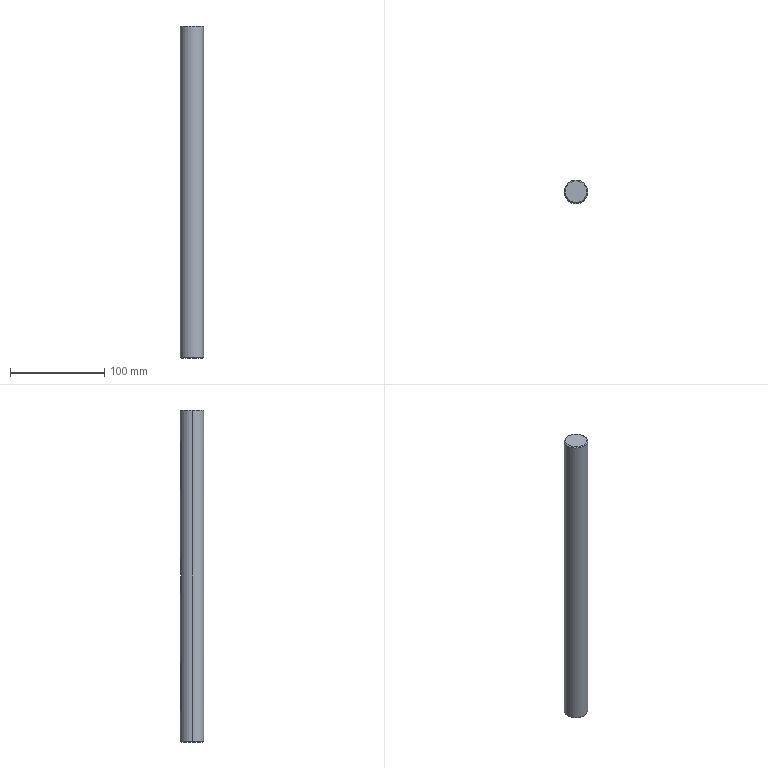Part | 1 solid | 35 faces | box 25 x 25 x 353 mm | volume 169122 mm3 | plane 17 | cylinder 14 | cone 4 | commonest cylinder face diameters 0.6 x12 25 x2
STEP:
#1=CARTESIAN_POINT('',(11.5,0.,176.5));
#2=VERTEX_POINT('',#1);
#3=CARTESIAN_POINT('',(-11.5,0.,176.5));
#4=VERTEX_POINT('',#3);
#5=CARTESIAN_POINT('',(0.,0.,176.5));
#6=DIRECTION('',(0.,0.,1.));
#7=DIRECTION('',(1.,0.,0.));
#8=AXIS2_PLACEMENT_3D('',#5,#6,#7);
#9=CIRCLE('',#8,11.5);
#10=EDGE_CURVE('',#2,#4,#9,.T.);
#11=ORIENTED_EDGE('',*,*,#10,.F.);
#12=CARTESIAN_POINT('',(12.5,0.,175.5));
#13=VERTEX_POINT('',#12);
#14=CARTESIAN_POINT('',(11.5,0.,176.5));
#15=DIRECTION('',(0.7071,0.,-0.7071));
#16=VECTOR('',#15,1000.);
#17=LINE('',#14,#16);
#18=EDGE_CURVE('',#2,#13,#17,.T.);
#19=ORIENTED_EDGE('',*,*,#18,.T.);
#20=CARTESIAN_POINT('',(-12.5,0.,175.5));
#21=VERTEX_POINT('',#20);
#22=CARTESIAN_POINT('',(0.,0.,175.5));
#23=DIRECTION('',(0.,0.,-1.));
#24=DIRECTION('',(1.,0.,0.));
#25=AXIS2_PLACEMENT_3D('',#22,#23,#24);
#26=CIRCLE('',#25,12.5);
#27=EDGE_CURVE('',#21,#13,#26,.T.);
#28=ORIENTED_EDGE('',*,*,#27,.F.);
#29=CARTESIAN_POINT('',(-11.5,0.,176.5));
#30=DIRECTION('',(-0.7071,0.,-0.7071));
#31=VECTOR('',#30,1000.);
#32=LINE('',#29,#31);
#33=EDGE_CURVE('',#4,#21,#32,.T.);
#34=ORIENTED_EDGE('',*,*,#33,.F.);
#35=EDGE_LOOP('',(#11,#19,#28,#34));
#36=FACE_OUTER_BOUND('',#35,.T.);
#37=CARTESIAN_POINT('',(0.,0.,176.5));
#38=DIRECTION('',(0.,0.,-1.));
#39=DIRECTION('',(-1.,0.,0.));
#40=AXIS2_PLACEMENT_3D('',#37,#38,#39);
#41=CONICAL_SURFACE('',#40,11.5,0.7854);
#42=ADVANCED_FACE('',(#36),#41,.T.);
#43=CARTESIAN_POINT('',(-11.5,0.,-176.5));
#44=VERTEX_POINT('',#43);
#45=CARTESIAN_POINT('',(11.5,0.,-176.5));
#46=VERTEX_POINT('',#45);
#47=CARTESIAN_POINT('',(0.,0.,-176.5));
#48=DIRECTION('',(0.,0.,-1.));
#49=DIRECTION('',(1.,0.,0.));
#50=AXIS2_PLACEMENT_3D('',#47,#48,#49);
#51=CIRCLE('',#50,11.5);
#52=EDGE_CURVE('',#44,#46,#51,.T.);
#53=ORIENTED_EDGE('',*,*,#52,.F.);
#54=CARTESIAN_POINT('',(-12.5,0.,-175.5));
#55=VERTEX_POINT('',#54);
#56=CARTESIAN_POINT('',(-12.5,0.,-175.5));
#57=DIRECTION('',(-0.7071,0.,0.7071));
#58=VECTOR('',#57,1000.);
#59=LINE('',#56,#58);
#60=EDGE_CURVE('',#44,#55,#59,.T.);
#61=ORIENTED_EDGE('',*,*,#60,.T.);
#62=CARTESIAN_POINT('',(12.5,0.,-175.5));
#63=VERTEX_POINT('',#62);
#64=CARTESIAN_POINT('',(0.,0.,-175.5));
#65=DIRECTION('',(0.,0.,1.));
#66=DIRECTION('',(1.,0.,0.));
#67=AXIS2_PLACEMENT_3D('',#64,#65,#66);
#68=CIRCLE('',#67,12.5);
#69=EDGE_CURVE('',#63,#55,#68,.T.);
#70=ORIENTED_EDGE('',*,*,#69,.F.);
#71=CARTESIAN_POINT('',(12.5,0.,-175.5));
#72=DIRECTION('',(0.7071,0.,0.7071));
#73=VECTOR('',#72,1000.);
#74=LINE('',#71,#73);
#75=EDGE_CURVE('',#46,#63,#74,.T.);
#76=ORIENTED_EDGE('',*,*,#75,.F.);
#77=EDGE_LOOP('',(#53,#61,#70,#76));
#78=FACE_OUTER_BOUND('',#77,.T.);
#79=CARTESIAN_POINT('',(0.,0.,-175.5));
#80=DIRECTION('',(0.,0.,1.));
#81=DIRECTION('',(1.,0.,0.));
#82=AXIS2_PLACEMENT_3D('',#79,#80,#81);
#83=CONICAL_SURFACE('',#82,12.5,0.7854);
#84=ADVANCED_FACE('',(#78),#83,.T.);
#85=CARTESIAN_POINT('',(-4.,11.843,143.5));
#86=VERTEX_POINT('',#85);
#87=CARTESIAN_POINT('',(-4.,11.843,93.5));
#88=VERTEX_POINT('',#87);
#89=CARTESIAN_POINT('',(-4.,11.843,176.5));
#90=DIRECTION('',(0.,0.,-1.));
#91=VECTOR('',#90,1000.);
#92=LINE('',#89,#91);
#93=EDGE_CURVE('',#86,#88,#92,.T.);
#94=ORIENTED_EDGE('',*,*,#93,.T.);
#95=CARTESIAN_POINT('',(4.,11.843,93.5));
#96=VERTEX_POINT('',#95);
#97=CARTESIAN_POINT('',(0.,0.,93.5));
#98=DIRECTION('',(0.,0.,-1.));
#99=DIRECTION('',(-1.,0.,0.));
#100=AXIS2_PLACEMENT_3D('',#97,#98,#99);
#101=CIRCLE('',#100,12.5);
#102=EDGE_CURVE('',#88,#96,#101,.T.);
#103=ORIENTED_EDGE('',*,*,#102,.T.);
#104=CARTESIAN_POINT('',(4.,11.843,143.5));
#105=VERTEX_POINT('',#104);
#106=CARTESIAN_POINT('',(4.,11.843,176.5));
#107=DIRECTION('',(0.,0.,1.));
#108=VECTOR('',#107,1000.);
#109=LINE('',#106,#108);
#110=EDGE_CURVE('',#96,#105,#109,.T.);
#111=ORIENTED_EDGE('',*,*,#110,.T.);
#112=CARTESIAN_POINT('',(0.,0.,143.5));
#113=DIRECTION('',(0.,0.,1.));
#114=DIRECTION('',(1.,0.,0.));
#115=AXIS2_PLACEMENT_3D('',#112,#113,#114);
#116=CIRCLE('',#115,12.5);
#117=EDGE_CURVE('',#105,#86,#116,.T.);
#118=ORIENTED_EDGE('',*,*,#117,.T.);
#119=EDGE_LOOP('',(#94,#103,#111,#118));
#120=FACE_BOUND('',#119,.T.);
#121=CARTESIAN_POINT('',(4.,11.843,-143.5));
#122=VERTEX_POINT('',#121);
#123=CARTESIAN_POINT('',(4.,11.843,-93.5));
#124=VERTEX_POINT('',#123);
#125=CARTESIAN_POINT('',(4.,11.843,176.5));
#126=DIRECTION('',(0.,0.,1.));
#127=VECTOR('',#126,1000.);
#128=LINE('',#125,#127);
#129=EDGE_CURVE('',#122,#124,#128,.T.);
#130=ORIENTED_EDGE('',*,*,#129,.T.);
#131=CARTESIAN_POINT('',(-4.,11.843,-93.5));
#132=VERTEX_POINT('',#131);
#133=CARTESIAN_POINT('',(0.,0.,-93.5));
#134=DIRECTION('',(0.,0.,1.));
#135=DIRECTION('',(1.,0.,0.));
#136=AXIS2_PLACEMENT_3D('',#133,#134,#135);
#137=CIRCLE('',#136,12.5);
#138=EDGE_CURVE('',#124,#132,#137,.T.);
#139=ORIENTED_EDGE('',*,*,#138,.T.);
#140=CARTESIAN_POINT('',(-4.,11.843,-143.5));
#141=VERTEX_POINT('',#140);
#142=CARTESIAN_POINT('',(-4.,11.843,176.5));
#143=DIRECTION('',(0.,0.,-1.));
#144=VECTOR('',#143,1000.);
#145=LINE('',#142,#144);
#146=EDGE_CURVE('',#132,#141,#145,.T.);
#147=ORIENTED_EDGE('',*,*,#146,.T.);
#148=CARTESIAN_POINT('',(0.,0.,-143.5));
#149=DIRECTION('',(0.,0.,-1.));
#150=DIRECTION('',(-1.,0.,0.));
#151=AXIS2_PLACEMENT_3D('',#148,#149,#150);
#152=CIRCLE('',#151,12.5);
#153=EDGE_CURVE('',#141,#122,#152,.T.);
#154=ORIENTED_EDGE('',*,*,#153,.T.);
#155=EDGE_LOOP('',(#130,#139,#147,#154));
#156=FACE_BOUND('',#155,.T.);
#157=CARTESIAN_POINT('',(4.,11.843,-17.5));
#158=VERTEX_POINT('',#157);
#159=CARTESIAN_POINT('',(4.,11.843,17.5));
#160=VERTEX_POINT('',#159);
#161=CARTESIAN_POINT('',(4.,11.843,176.5));
#162=DIRECTION('',(0.,0.,1.));
#163=VECTOR('',#162,1000.);
#164=LINE('',#161,#163);
#165=EDGE_CURVE('',#158,#160,#164,.T.);
#166=ORIENTED_EDGE('',*,*,#165,.T.);
#167=CARTESIAN_POINT('',(-4.,11.843,17.5));
#168=VERTEX_POINT('',#167);
#169=CARTESIAN_POINT('',(0.,0.,17.5));
#170=DIRECTION('',(0.,0.,1.));
#171=DIRECTION('',(1.,0.,0.));
#172=AXIS2_PLACEMENT_3D('',#169,#170,#171);
#173=CIRCLE('',#172,12.5);
#174=EDGE_CURVE('',#160,#168,#173,.T.);
#175=ORIENTED_EDGE('',*,*,#174,.T.);
#176=CARTESIAN_POINT('',(-4.,11.843,-17.5));
#177=VERTEX_POINT('',#176);
#178=CARTESIAN_POINT('',(-4.,11.843,176.5));
#179=DIRECTION('',(0.,0.,-1.));
#180=VECTOR('',#179,1000.);
#181=LINE('',#178,#180);
#182=EDGE_CURVE('',#168,#177,#181,.T.);
#183=ORIENTED_EDGE('',*,*,#182,.T.);
#184=CARTESIAN_POINT('',(0.,0.,-17.5));
#185=DIRECTION('',(0.,0.,-1.));
#186=DIRECTION('',(-1.,0.,0.));
#187=AXIS2_PLACEMENT_3D('',#184,#185,#186);
#188=CIRCLE('',#187,12.5);
#189=EDGE_CURVE('',#177,#158,#188,.T.);
#190=ORIENTED_EDGE('',*,*,#189,.T.);
#191=EDGE_LOOP('',(#166,#175,#183,#190));
#192=FACE_BOUND('',#191,.T.);
#193=ORIENTED_EDGE('',*,*,#27,.T.);
#194=CARTESIAN_POINT('',(12.5,0.,176.5));
#195=DIRECTION('',(0.,0.,-1.));
#196=VECTOR('',#195,1000.);
#197=LINE('',#194,#196);
#198=EDGE_CURVE('',#13,#63,#197,.T.);
#199=ORIENTED_EDGE('',*,*,#198,.T.);
#200=ORIENTED_EDGE('',*,*,#69,.T.);
#201=CARTESIAN_POINT('',(-12.5,0.,176.5));
#202=DIRECTION('',(0.,0.,-1.));
#203=VECTOR('',#202,1000.);
#204=LINE('',#201,#203);
#205=EDGE_CURVE('',#21,#55,#204,.T.);
#206=ORIENTED_EDGE('',*,*,#205,.F.);
#207=EDGE_LOOP('',(#193,#199,#200,#206));
#208=FACE_OUTER_BOUND('',#207,.T.);
#209=CARTESIAN_POINT('',(0.,0.,176.5));
#210=DIRECTION('',(0.,0.,-1.));
#211=DIRECTION('',(-1.,0.,0.));
#212=AXIS2_PLACEMENT_3D('',#209,#210,#211);
#213=CYLINDRICAL_SURFACE('',#212,12.5);
#214=ADVANCED_FACE('',(#120,#156,#192,#208),#213,.T.);
#215=ORIENTED_EDGE('',*,*,#198,.F.);
#216=CARTESIAN_POINT('',(0.,0.,175.5));
#217=DIRECTION('',(0.,0.,-1.));
#218=DIRECTION('',(1.,0.,0.));
#219=AXIS2_PLACEMENT_3D('',#216,#217,#218);
#220=CIRCLE('',#219,12.5);
#221=EDGE_CURVE('',#13,#21,#220,.T.);
#222=ORIENTED_EDGE('',*,*,#221,.T.);
#223=ORIENTED_EDGE('',*,*,#205,.T.);
#224=CARTESIAN_POINT('',(0.,0.,-175.5));
#225=DIRECTION('',(0.,0.,1.));
#226=DIRECTION('',(1.,0.,0.));
#227=AXIS2_PLACEMENT_3D('',#224,#225,#226);
#228=CIRCLE('',#227,12.5);
#229=EDGE_CURVE('',#55,#63,#228,.T.);
#230=ORIENTED_EDGE('',*,*,#229,.T.);
#231=EDGE_LOOP('',(#215,#222,#223,#230));
#232=FACE_OUTER_BOUND('',#231,.T.);
#233=CARTESIAN_POINT('',(0.,0.,176.5));
#234=DIRECTION('',(0.,0.,-1.));
#235=DIRECTION('',(-1.,0.,0.));
#236=AXIS2_PLACEMENT_3D('',#233,#234,#235);
#237=CYLINDRICAL_SURFACE('',#236,12.5);
#238=ADVANCED_FACE('',(#232),#237,.T.);
#239=CARTESIAN_POINT('',(0.,0.,176.5));
#240=DIRECTION('',(0.,0.,1.));
#241=DIRECTION('',(1.,0.,0.));
#242=AXIS2_PLACEMENT_3D('',#239,#240,#241);
#243=CIRCLE('',#242,11.5);
#244=EDGE_CURVE('',#4,#2,#243,.T.);
#245=ORIENTED_EDGE('',*,*,#244,.T.);
#246=ORIENTED_EDGE('',*,*,#10,.T.);
#247=EDGE_LOOP('',(#245,#246));
#248=FACE_OUTER_BOUND('',#247,.T.);
#249=CARTESIAN_POINT('',(0.,0.,176.5));
#250=DIRECTION('',(0.,0.,1.));
#251=DIRECTION('',(1.,0.,0.));
#252=AXIS2_PLACEMENT_3D('',#249,#250,#251);
#253=PLANE('',#252);
#254=ADVANCED_FACE('',(#248),#253,.T.);
#255=CARTESIAN_POINT('',(0.,0.,-176.5));
#256=DIRECTION('',(0.,0.,-1.));
#257=DIRECTION('',(1.,0.,0.));
#258=AXIS2_PLACEMENT_3D('',#255,#256,#257);
#259=CIRCLE('',#258,11.5);
#260=EDGE_CURVE('',#46,#44,#259,.T.);
#261=ORIENTED_EDGE('',*,*,#260,.T.);
#262=ORIENTED_EDGE('',*,*,#52,.T.);
#263=EDGE_LOOP('',(#261,#262));
#264=FACE_OUTER_BOUND('',#263,.T.);
#265=CARTESIAN_POINT('',(0.,0.,-176.5));
#266=DIRECTION('',(0.,0.,1.));
#267=DIRECTION('',(1.,0.,0.));
#268=AXIS2_PLACEMENT_3D('',#265,#266,#267);
#269=PLANE('',#268);
#270=ADVANCED_FACE('',(#264),#269,.F.);
#271=CARTESIAN_POINT('',(-4.,8.8,17.5));
#272=VERTEX_POINT('',#271);
#273=CARTESIAN_POINT('',(-4.,8.5,17.5));
#274=DIRECTION('',(0.,1.,0.));
#275=VECTOR('',#274,1000.);
#276=LINE('',#273,#275);
#277=EDGE_CURVE('',#272,#168,#276,.T.);
#278=ORIENTED_EDGE('',*,*,#277,.F.);
#279=CARTESIAN_POINT('',(-4.,8.8,-17.5));
#280=VERTEX_POINT('',#279);
#281=CARTESIAN_POINT('',(-4.,8.8,-17.5));
#282=DIRECTION('',(0.,0.,-1.));
#283=VECTOR('',#282,1000.);
#284=LINE('',#281,#283);
#285=EDGE_CURVE('',#272,#280,#284,.T.);
#286=ORIENTED_EDGE('',*,*,#285,.T.);
#287=CARTESIAN_POINT('',(-4.,8.5,-17.5));
#288=DIRECTION('',(0.,1.,0.));
#289=VECTOR('',#288,1000.);
#290=LINE('',#287,#289);
#291=EDGE_CURVE('',#280,#177,#290,.T.);
#292=ORIENTED_EDGE('',*,*,#291,.T.);
#293=ORIENTED_EDGE('',*,*,#182,.F.);
#294=EDGE_LOOP('',(#278,#286,#292,#293));
#295=FACE_OUTER_BOUND('',#294,.T.);
#296=CARTESIAN_POINT('',(-4.,8.5,-17.5));
#297=DIRECTION('',(-1.,0.,0.));
#298=DIRECTION('',(0.,0.,1.));
#299=AXIS2_PLACEMENT_3D('',#296,#297,#298);
#300=PLANE('',#299);
#301=ADVANCED_FACE('',(#295),#300,.F.);
#302=ORIENTED_EDGE('',*,*,#291,.F.);
#303=CARTESIAN_POINT('',(4.,8.8,-17.5));
#304=VERTEX_POINT('',#303);
#305=CARTESIAN_POINT('',(-4.,8.8,-17.5));
#306=DIRECTION('',(1.,0.,0.));
#307=VECTOR('',#306,1000.);
#308=LINE('',#305,#307);
#309=EDGE_CURVE('',#280,#304,#308,.T.);
#310=ORIENTED_EDGE('',*,*,#309,.T.);
#311=CARTESIAN_POINT('',(4.,8.5,-17.5));
#312=DIRECTION('',(0.,1.,0.));
#313=VECTOR('',#312,1000.);
#314=LINE('',#311,#313);
#315=EDGE_CURVE('',#304,#158,#314,.T.);
#316=ORIENTED_EDGE('',*,*,#315,.T.);
#317=ORIENTED_EDGE('',*,*,#189,.F.);
#318=EDGE_LOOP('',(#302,#310,#316,#317));
#319=FACE_OUTER_BOUND('',#318,.T.);
#320=CARTESIAN_POINT('',(-4.,8.5,-17.5));
#321=DIRECTION('',(0.,0.,-1.));
#322=DIRECTION('',(-1.,0.,0.));
#323=AXIS2_PLACEMENT_3D('',#320,#321,#322);
#324=PLANE('',#323);
#325=ADVANCED_FACE('',(#319),#324,.F.);
#326=ORIENTED_EDGE('',*,*,#315,.F.);
#327=CARTESIAN_POINT('',(4.,8.8,17.5));
#328=VERTEX_POINT('',#327);
#329=CARTESIAN_POINT('',(4.,8.8,-17.5));
#330=DIRECTION('',(0.,0.,1.));
#331=VECTOR('',#330,1000.);
#332=LINE('',#329,#331);
#333=EDGE_CURVE('',#304,#328,#332,.T.);
#334=ORIENTED_EDGE('',*,*,#333,.T.);
#335=CARTESIAN_POINT('',(4.,8.5,17.5));
#336=DIRECTION('',(0.,1.,0.));
#337=VECTOR('',#336,1000.);
#338=LINE('',#335,#337);
#339=EDGE_CURVE('',#328,#160,#338,.T.);
#340=ORIENTED_EDGE('',*,*,#339,.T.);
#341=ORIENTED_EDGE('',*,*,#165,.F.);
#342=EDGE_LOOP('',(#326,#334,#340,#341));
#343=FACE_OUTER_BOUND('',#342,.T.);
#344=CARTESIAN_POINT('',(4.,8.5,-17.5));
#345=DIRECTION('',(1.,0.,0.));
#346=DIRECTION('',(0.,0.,-1.));
#347=AXIS2_PLACEMENT_3D('',#344,#345,#346);
#348=PLANE('',#347);
#349=ADVANCED_FACE('',(#343),#348,.F.);
#350=ORIENTED_EDGE('',*,*,#339,.F.);
#351=CARTESIAN_POINT('',(-4.,8.8,17.5));
#352=DIRECTION('',(-1.,0.,0.));
#353=VECTOR('',#352,1000.);
#354=LINE('',#351,#353);
#355=EDGE_CURVE('',#328,#272,#354,.T.);
#356=ORIENTED_EDGE('',*,*,#355,.T.);
#357=ORIENTED_EDGE('',*,*,#277,.T.);
#358=ORIENTED_EDGE('',*,*,#174,.F.);
#359=EDGE_LOOP('',(#350,#356,#357,#358));
#360=FACE_OUTER_BOUND('',#359,.T.);
#361=CARTESIAN_POINT('',(-4.,8.5,17.5));
#362=DIRECTION('',(0.,0.,1.));
#363=DIRECTION('',(1.,0.,0.));
#364=AXIS2_PLACEMENT_3D('',#361,#362,#363);
#365=PLANE('',#364);
#366=ADVANCED_FACE('',(#360),#365,.F.);
#367=CARTESIAN_POINT('',(-3.7,8.5,17.2));
#368=VERTEX_POINT('',#367);
#369=CARTESIAN_POINT('',(3.7,8.5,17.2));
#370=VERTEX_POINT('',#369);
#371=CARTESIAN_POINT('',(0.,8.5,17.2));
#372=DIRECTION('',(1.,0.,0.));
#373=VECTOR('',#372,1000.);
#374=LINE('',#371,#373);
#375=EDGE_CURVE('',#368,#370,#374,.T.);
#376=ORIENTED_EDGE('',*,*,#375,.T.);
#377=CARTESIAN_POINT('',(3.7,8.5,-17.2));
#378=VERTEX_POINT('',#377);
#379=CARTESIAN_POINT('',(3.7,8.5,0.));
#380=DIRECTION('',(0.,0.,-1.));
#381=VECTOR('',#380,1000.);
#382=LINE('',#379,#381);
#383=EDGE_CURVE('',#370,#378,#382,.T.);
#384=ORIENTED_EDGE('',*,*,#383,.T.);
#385=CARTESIAN_POINT('',(-3.7,8.5,-17.2));
#386=VERTEX_POINT('',#385);
#387=CARTESIAN_POINT('',(0.,8.5,-17.2));
#388=DIRECTION('',(-1.,0.,0.));
#389=VECTOR('',#388,1000.);
#390=LINE('',#387,#389);
#391=EDGE_CURVE('',#378,#386,#390,.T.);
#392=ORIENTED_EDGE('',*,*,#391,.T.);
#393=CARTESIAN_POINT('',(-3.7,8.5,0.));
#394=DIRECTION('',(0.,0.,1.));
#395=VECTOR('',#394,1000.);
#396=LINE('',#393,#395);
#397=EDGE_CURVE('',#386,#368,#396,.T.);
#398=ORIENTED_EDGE('',*,*,#397,.T.);
#399=EDGE_LOOP('',(#376,#384,#392,#398));
#400=FACE_OUTER_BOUND('',#399,.T.);
#401=CARTESIAN_POINT('',(0.,8.5,0.));
#402=DIRECTION('',(0.,1.,0.));
#403=DIRECTION('',(0.,0.,1.));
#404=AXIS2_PLACEMENT_3D('',#401,#402,#403);
#405=PLANE('',#404);
#406=ADVANCED_FACE('',(#400),#405,.T.);
#407=CARTESIAN_POINT('',(-4.,8.8,-93.5));
#408=VERTEX_POINT('',#407);
#409=CARTESIAN_POINT('',(-4.,8.5,-93.5));
#410=DIRECTION('',(0.,1.,0.));
#411=VECTOR('',#410,1000.);
#412=LINE('',#409,#411);
#413=EDGE_CURVE('',#408,#132,#412,.T.);
#414=ORIENTED_EDGE('',*,*,#413,.F.);
#415=CARTESIAN_POINT('',(-4.,8.8,-143.5));
#416=VERTEX_POINT('',#415);
#417=CARTESIAN_POINT('',(-4.,8.8,-143.5));
#418=DIRECTION('',(0.,0.,-1.));
#419=VECTOR('',#418,1000.);
#420=LINE('',#417,#419);
#421=EDGE_CURVE('',#408,#416,#420,.T.);
#422=ORIENTED_EDGE('',*,*,#421,.T.);
#423=CARTESIAN_POINT('',(-4.,8.5,-143.5));
#424=DIRECTION('',(0.,1.,0.));
#425=VECTOR('',#424,1000.);
#426=LINE('',#423,#425);
#427=EDGE_CURVE('',#416,#141,#426,.T.);
#428=ORIENTED_EDGE('',*,*,#427,.T.);
#429=ORIENTED_EDGE('',*,*,#146,.F.);
#430=EDGE_LOOP('',(#414,#422,#428,#429));
#431=FACE_OUTER_BOUND('',#430,.T.);
#432=CARTESIAN_POINT('',(-4.,8.5,-143.5));
#433=DIRECTION('',(-1.,0.,0.));
#434=DIRECTION('',(0.,0.,1.));
#435=AXIS2_PLACEMENT_3D('',#432,#433,#434);
#436=PLANE('',#435);
#437=ADVANCED_FACE('',(#431),#436,.F.);
#438=ORIENTED_EDGE('',*,*,#427,.F.);
#439=CARTESIAN_POINT('',(4.,8.8,-143.5));
#440=VERTEX_POINT('',#439);
#441=CARTESIAN_POINT('',(-4.,8.8,-143.5));
#442=DIRECTION('',(1.,0.,0.));
#443=VECTOR('',#442,1000.);
#444=LINE('',#441,#443);
#445=EDGE_CURVE('',#416,#440,#444,.T.);
#446=ORIENTED_EDGE('',*,*,#445,.T.);
#447=CARTESIAN_POINT('',(4.,8.5,-143.5));
#448=DIRECTION('',(0.,1.,0.));
#449=VECTOR('',#448,1000.);
#450=LINE('',#447,#449);
#451=EDGE_CURVE('',#440,#122,#450,.T.);
#452=ORIENTED_EDGE('',*,*,#451,.T.);
#453=ORIENTED_EDGE('',*,*,#153,.F.);
#454=EDGE_LOOP('',(#438,#446,#452,#453));
#455=FACE_OUTER_BOUND('',#454,.T.);
#456=CARTESIAN_POINT('',(-4.,8.5,-143.5));
#457=DIRECTION('',(0.,0.,-1.));
#458=DIRECTION('',(-1.,0.,0.));
#459=AXIS2_PLACEMENT_3D('',#456,#457,#458);
#460=PLANE('',#459);
#461=ADVANCED_FACE('',(#455),#460,.F.);
#462=ORIENTED_EDGE('',*,*,#451,.F.);
#463=CARTESIAN_POINT('',(4.,8.8,-93.5));
#464=VERTEX_POINT('',#463);
#465=CARTESIAN_POINT('',(4.,8.8,-143.5));
#466=DIRECTION('',(0.,0.,1.));
#467=VECTOR('',#466,1000.);
#468=LINE('',#465,#467);
#469=EDGE_CURVE('',#440,#464,#468,.T.);
#470=ORIENTED_EDGE('',*,*,#469,.T.);
#471=CARTESIAN_POINT('',(4.,8.5,-93.5));
#472=DIRECTION('',(0.,1.,0.));
#473=VECTOR('',#472,1000.);
#474=LINE('',#471,#473);
#475=EDGE_CURVE('',#464,#124,#474,.T.);
#476=ORIENTED_EDGE('',*,*,#475,.T.);
#477=ORIENTED_EDGE('',*,*,#129,.F.);
#478=EDGE_LOOP('',(#462,#470,#476,#477));
#479=FACE_OUTER_BOUND('',#478,.T.);
#480=CARTESIAN_POINT('',(4.,8.5,-143.5));
#481=DIRECTION('',(1.,0.,0.));
#482=DIRECTION('',(0.,0.,-1.));
#483=AXIS2_PLACEMENT_3D('',#480,#481,#482);
#484=PLANE('',#483);
#485=ADVANCED_FACE('',(#479),#484,.F.);
#486=ORIENTED_EDGE('',*,*,#475,.F.);
#487=CARTESIAN_POINT('',(-4.,8.8,-93.5));
#488=DIRECTION('',(-1.,0.,0.));
#489=VECTOR('',#488,1000.);
#490=LINE('',#487,#489);
#491=EDGE_CURVE('',#464,#408,#490,.T.);
#492=ORIENTED_EDGE('',*,*,#491,.T.);
#493=ORIENTED_EDGE('',*,*,#413,.T.);
#494=ORIENTED_EDGE('',*,*,#138,.F.);
#495=EDGE_LOOP('',(#486,#492,#493,#494));
#496=FACE_OUTER_BOUND('',#495,.T.);
#497=CARTESIAN_POINT('',(-4.,8.5,-93.5));
#498=DIRECTION('',(0.,0.,1.));
#499=DIRECTION('',(1.,0.,0.));
#500=AXIS2_PLACEMENT_3D('',#497,#498,#499);
#501=PLANE('',#500);
#502=ADVANCED_FACE('',(#496),#501,.F.);
#503=CARTESIAN_POINT('',(-3.7,8.5,-143.2));
#504=VERTEX_POINT('',#503);
#505=CARTESIAN_POINT('',(-3.7,8.5,-93.8));
#506=VERTEX_POINT('',#505);
#507=CARTESIAN_POINT('',(-3.7,8.5,0.));
#508=DIRECTION('',(0.,0.,1.));
#509=VECTOR('',#508,1000.);
#510=LINE('',#507,#509);
#511=EDGE_CURVE('',#504,#506,#510,.T.);
#512=ORIENTED_EDGE('',*,*,#511,.T.);
#513=CARTESIAN_POINT('',(3.7,8.5,-93.8));
#514=VERTEX_POINT('',#513);
#515=CARTESIAN_POINT('',(0.,8.5,-93.8));
#516=DIRECTION('',(1.,0.,0.));
#517=VECTOR('',#516,1000.);
#518=LINE('',#515,#517);
#519=EDGE_CURVE('',#506,#514,#518,.T.);
#520=ORIENTED_EDGE('',*,*,#519,.T.);
#521=CARTESIAN_POINT('',(3.7,8.5,-143.2));
#522=VERTEX_POINT('',#521);
#523=CARTESIAN_POINT('',(3.7,8.5,0.));
#524=DIRECTION('',(0.,0.,-1.));
#525=VECTOR('',#524,1000.);
#526=LINE('',#523,#525);
#527=EDGE_CURVE('',#514,#522,#526,.T.);
#528=ORIENTED_EDGE('',*,*,#527,.T.);
#529=CARTESIAN_POINT('',(0.,8.5,-143.2));
#530=DIRECTION('',(-1.,0.,0.));
#531=VECTOR('',#530,1000.);
#532=LINE('',#529,#531);
#533=EDGE_CURVE('',#522,#504,#532,.T.);
#534=ORIENTED_EDGE('',*,*,#533,.T.);
#535=EDGE_LOOP('',(#512,#520,#528,#534));
#536=FACE_OUTER_BOUND('',#535,.T.);
#537=CARTESIAN_POINT('',(0.,8.5,0.));
#538=DIRECTION('',(0.,1.,0.));
#539=DIRECTION('',(0.,0.,1.));
#540=AXIS2_PLACEMENT_3D('',#537,#538,#539);
#541=PLANE('',#540);
#542=ADVANCED_FACE('',(#536),#541,.T.);
#543=CARTESIAN_POINT('',(4.,8.8,143.5));
#544=VERTEX_POINT('',#543);
#545=CARTESIAN_POINT('',(4.,8.5,143.5));
#546=DIRECTION('',(0.,1.,0.));
#547=VECTOR('',#546,1000.);
#548=LINE('',#545,#547);
#549=EDGE_CURVE('',#544,#105,#548,.T.);
#550=ORIENTED_EDGE('',*,*,#549,.F.);
#551=CARTESIAN_POINT('',(-4.,8.8,143.5));
#552=VERTEX_POINT('',#551);
#553=CARTESIAN_POINT('',(-4.,8.8,143.5));
#554=DIRECTION('',(-1.,0.,0.));
#555=VECTOR('',#554,1000.);
#556=LINE('',#553,#555);
#557=EDGE_CURVE('',#544,#552,#556,.T.);
#558=ORIENTED_EDGE('',*,*,#557,.T.);
#559=CARTESIAN_POINT('',(-4.,8.5,143.5));
#560=DIRECTION('',(0.,1.,0.));
#561=VECTOR('',#560,1000.);
#562=LINE('',#559,#561);
#563=EDGE_CURVE('',#552,#86,#562,.T.);
#564=ORIENTED_EDGE('',*,*,#563,.T.);
#565=ORIENTED_EDGE('',*,*,#117,.F.);
#566=EDGE_LOOP('',(#550,#558,#564,#565));
#567=FACE_OUTER_BOUND('',#566,.T.);
#568=CARTESIAN_POINT('',(-4.,8.5,143.5));
#569=DIRECTION('',(0.,0.,1.));
#570=DIRECTION('',(1.,0.,0.));
#571=AXIS2_PLACEMENT_3D('',#568,#569,#570);
#572=PLANE('',#571);
#573=ADVANCED_FACE('',(#567),#572,.F.);
#574=ORIENTED_EDGE('',*,*,#563,.F.);
#575=CARTESIAN_POINT('',(-4.,8.8,93.5));
#576=VERTEX_POINT('',#575);
#577=CARTESIAN_POINT('',(-4.,8.8,143.5));
#578=DIRECTION('',(0.,0.,-1.));
#579=VECTOR('',#578,1000.);
#580=LINE('',#577,#579);
#581=EDGE_CURVE('',#552,#576,#580,.T.);
#582=ORIENTED_EDGE('',*,*,#581,.T.);
#583=CARTESIAN_POINT('',(-4.,8.5,93.5));
#584=DIRECTION('',(0.,1.,0.));
#585=VECTOR('',#584,1000.);
#586=LINE('',#583,#585);
#587=EDGE_CURVE('',#576,#88,#586,.T.);
#588=ORIENTED_EDGE('',*,*,#587,.T.);
#589=ORIENTED_EDGE('',*,*,#93,.F.);
#590=EDGE_LOOP('',(#574,#582,#588,#589));
#591=FACE_OUTER_BOUND('',#590,.T.);
#592=CARTESIAN_POINT('',(-4.,8.5,143.5));
#593=DIRECTION('',(-1.,0.,0.));
#594=DIRECTION('',(0.,0.,1.));
#595=AXIS2_PLACEMENT_3D('',#592,#593,#594);
#596=PLANE('',#595);
#597=ADVANCED_FACE('',(#591),#596,.F.);
#598=ORIENTED_EDGE('',*,*,#587,.F.);
#599=CARTESIAN_POINT('',(4.,8.8,93.5));
#600=VERTEX_POINT('',#599);
#601=CARTESIAN_POINT('',(-4.,8.8,93.5));
#602=DIRECTION('',(1.,0.,0.));
#603=VECTOR('',#602,1000.);
#604=LINE('',#601,#603);
#605=EDGE_CURVE('',#576,#600,#604,.T.);
#606=ORIENTED_EDGE('',*,*,#605,.T.);
#607=CARTESIAN_POINT('',(4.,8.5,93.5));
#608=DIRECTION('',(0.,1.,0.));
#609=VECTOR('',#608,1000.);
#610=LINE('',#607,#609);
#611=EDGE_CURVE('',#600,#96,#610,.T.);
#612=ORIENTED_EDGE('',*,*,#611,.T.);
#613=ORIENTED_EDGE('',*,*,#102,.F.);
#614=EDGE_LOOP('',(#598,#606,#612,#613));
#615=FACE_OUTER_BOUND('',#614,.T.);
#616=CARTESIAN_POINT('',(-4.,8.5,93.5));
#617=DIRECTION('',(0.,0.,-1.));
#618=DIRECTION('',(-1.,0.,0.));
#619=AXIS2_PLACEMENT_3D('',#616,#617,#618);
#620=PLANE('',#619);
#621=ADVANCED_FACE('',(#615),#620,.F.);
#622=ORIENTED_EDGE('',*,*,#611,.F.);
#623=CARTESIAN_POINT('',(4.,8.8,143.5));
#624=DIRECTION('',(0.,0.,1.));
#625=VECTOR('',#624,1000.);
#626=LINE('',#623,#625);
#627=EDGE_CURVE('',#600,#544,#626,.T.);
#628=ORIENTED_EDGE('',*,*,#627,.T.);
#629=ORIENTED_EDGE('',*,*,#549,.T.);
#630=ORIENTED_EDGE('',*,*,#110,.F.);
#631=EDGE_LOOP('',(#622,#628,#629,#630));
#632=FACE_OUTER_BOUND('',#631,.T.);
#633=CARTESIAN_POINT('',(4.,8.5,143.5));
#634=DIRECTION('',(1.,0.,0.));
#635=DIRECTION('',(0.,0.,-1.));
#636=AXIS2_PLACEMENT_3D('',#633,#634,#635);
#637=PLANE('',#636);
#638=ADVANCED_FACE('',(#632),#637,.F.);
#639=CARTESIAN_POINT('',(-3.7,8.5,93.8));
#640=VERTEX_POINT('',#639);
#641=CARTESIAN_POINT('',(-3.7,8.5,143.2));
#642=VERTEX_POINT('',#641);
#643=CARTESIAN_POINT('',(-3.7,8.5,0.));
#644=DIRECTION('',(0.,0.,1.));
#645=VECTOR('',#644,1000.);
#646=LINE('',#643,#645);
#647=EDGE_CURVE('',#640,#642,#646,.T.);
#648=ORIENTED_EDGE('',*,*,#647,.T.);
#649=CARTESIAN_POINT('',(3.7,8.5,143.2));
#650=VERTEX_POINT('',#649);
#651=CARTESIAN_POINT('',(0.,8.5,143.2));
#652=DIRECTION('',(1.,0.,0.));
#653=VECTOR('',#652,1000.);
#654=LINE('',#651,#653);
#655=EDGE_CURVE('',#642,#650,#654,.T.);
#656=ORIENTED_EDGE('',*,*,#655,.T.);
#657=CARTESIAN_POINT('',(3.7,8.5,93.8));
#658=VERTEX_POINT('',#657);
#659=CARTESIAN_POINT('',(3.7,8.5,0.));
#660=DIRECTION('',(0.,0.,-1.));
#661=VECTOR('',#660,1000.);
#662=LINE('',#659,#661);
#663=EDGE_CURVE('',#650,#658,#662,.T.);
#664=ORIENTED_EDGE('',*,*,#663,.T.);
#665=CARTESIAN_POINT('',(0.,8.5,93.8));
#666=DIRECTION('',(-1.,0.,0.));
#667=VECTOR('',#666,1000.);
#668=LINE('',#665,#667);
#669=EDGE_CURVE('',#658,#640,#668,.T.);
#670=ORIENTED_EDGE('',*,*,#669,.T.);
#671=EDGE_LOOP('',(#648,#656,#664,#670));
#672=FACE_OUTER_BOUND('',#671,.T.);
#673=CARTESIAN_POINT('',(0.,8.5,0.));
#674=DIRECTION('',(0.,1.,0.));
#675=DIRECTION('',(0.,0.,1.));
#676=AXIS2_PLACEMENT_3D('',#673,#674,#675);
#677=PLANE('',#676);
#678=ADVANCED_FACE('',(#672),#677,.T.);
#679=ORIENTED_EDGE('',*,*,#60,.F.);
#680=ORIENTED_EDGE('',*,*,#260,.F.);
#681=ORIENTED_EDGE('',*,*,#75,.T.);
#682=ORIENTED_EDGE('',*,*,#229,.F.);
#683=EDGE_LOOP('',(#679,#680,#681,#682));
#684=FACE_OUTER_BOUND('',#683,.T.);
#685=CARTESIAN_POINT('',(0.,0.,-175.5));
#686=DIRECTION('',(0.,0.,1.));
#687=DIRECTION('',(1.,0.,0.));
#688=AXIS2_PLACEMENT_3D('',#685,#686,#687);
#689=CONICAL_SURFACE('',#688,12.5,0.7854);
#690=ADVANCED_FACE('',(#684),#689,.T.);
#691=ORIENTED_EDGE('',*,*,#18,.F.);
#692=ORIENTED_EDGE('',*,*,#244,.F.);
#693=ORIENTED_EDGE('',*,*,#33,.T.);
#694=ORIENTED_EDGE('',*,*,#221,.F.);
#695=EDGE_LOOP('',(#691,#692,#693,#694));
#696=FACE_OUTER_BOUND('',#695,.T.);
#697=CARTESIAN_POINT('',(0.,0.,176.5));
#698=DIRECTION('',(0.,0.,-1.));
#699=DIRECTION('',(-1.,0.,0.));
#700=AXIS2_PLACEMENT_3D('',#697,#698,#699);
#701=CONICAL_SURFACE('',#700,11.5,0.7854);
#702=ADVANCED_FACE('',(#696),#701,.T.);
#703=CARTESIAN_POINT('',(4.,8.8,93.5));
#704=CARTESIAN_POINT('',(4.,8.624,93.5));
#705=CARTESIAN_POINT('',(3.876,8.5,93.624));
#706=CARTESIAN_POINT('',(3.7,8.5,93.8));
#707=(BOUNDED_CURVE()B_SPLINE_CURVE(3,(#703,#704,#705,#706),.UNSPECIFIED.,.F.,.F.)B_SPLINE_CURVE_WITH_KNOTS((4,4),(0.,1.571),.UNSPECIFIED.)CURVE()GEOMETRIC_REPRESENTATION_ITEM()RATIONAL_B_SPLINE_CURVE((1.,0.8047,0.8047,1.))REPRESENTATION_ITEM(''));
#708=EDGE_CURVE('',#600,#658,#707,.T.);
#709=ORIENTED_EDGE('',*,*,#708,.F.);
#710=ORIENTED_EDGE('',*,*,#605,.F.);
#711=CARTESIAN_POINT('',(-3.7,8.5,93.8));
#712=CARTESIAN_POINT('',(-3.876,8.5,93.624));
#713=CARTESIAN_POINT('',(-4.,8.624,93.5));
#714=CARTESIAN_POINT('',(-4.,8.8,93.5));
#715=(BOUNDED_CURVE()B_SPLINE_CURVE(3,(#711,#712,#713,#714),.UNSPECIFIED.,.F.,.F.)B_SPLINE_CURVE_WITH_KNOTS((4,4),(4.712,6.283),.UNSPECIFIED.)CURVE()GEOMETRIC_REPRESENTATION_ITEM()RATIONAL_B_SPLINE_CURVE((1.,0.8047,0.8047,1.))REPRESENTATION_ITEM(''));
#716=EDGE_CURVE('',#640,#576,#715,.T.);
#717=ORIENTED_EDGE('',*,*,#716,.F.);
#718=ORIENTED_EDGE('',*,*,#669,.F.);
#719=EDGE_LOOP('',(#709,#710,#717,#718));
#720=FACE_OUTER_BOUND('',#719,.T.);
#721=CARTESIAN_POINT('',(0.,8.8,93.8));
#722=DIRECTION('',(-1.,0.,0.));
#723=DIRECTION('',(0.,0.,1.));
#724=AXIS2_PLACEMENT_3D('',#721,#722,#723);
#725=CYLINDRICAL_SURFACE('',#724,0.3);
#726=ADVANCED_FACE('',(#720),#725,.F.);
#727=ORIENTED_EDGE('',*,*,#716,.T.);
#728=ORIENTED_EDGE('',*,*,#581,.F.);
#729=CARTESIAN_POINT('',(-3.7,8.5,143.2));
#730=CARTESIAN_POINT('',(-3.876,8.5,143.376));
#731=CARTESIAN_POINT('',(-4.,8.624,143.5));
#732=CARTESIAN_POINT('',(-4.,8.8,143.5));
#733=(BOUNDED_CURVE()B_SPLINE_CURVE(3,(#729,#730,#731,#732),.UNSPECIFIED.,.F.,.F.)B_SPLINE_CURVE_WITH_KNOTS((4,4),(1.571,3.142),.UNSPECIFIED.)CURVE()GEOMETRIC_REPRESENTATION_ITEM()RATIONAL_B_SPLINE_CURVE((1.,0.8047,0.8047,1.))REPRESENTATION_ITEM(''));
#734=EDGE_CURVE('',#642,#552,#733,.T.);
#735=ORIENTED_EDGE('',*,*,#734,.F.);
#736=ORIENTED_EDGE('',*,*,#647,.F.);
#737=EDGE_LOOP('',(#727,#728,#735,#736));
#738=FACE_OUTER_BOUND('',#737,.T.);
#739=CARTESIAN_POINT('',(-3.7,8.8,0.));
#740=DIRECTION('',(0.,0.,1.));
#741=DIRECTION('',(1.,0.,0.));
#742=AXIS2_PLACEMENT_3D('',#739,#740,#741);
#743=CYLINDRICAL_SURFACE('',#742,0.3);
#744=ADVANCED_FACE('',(#738),#743,.F.);
#745=ORIENTED_EDGE('',*,*,#708,.T.);
#746=ORIENTED_EDGE('',*,*,#663,.F.);
#747=CARTESIAN_POINT('',(4.,8.8,143.5));
#748=CARTESIAN_POINT('',(4.,8.624,143.5));
#749=CARTESIAN_POINT('',(3.876,8.5,143.376));
#750=CARTESIAN_POINT('',(3.7,8.5,143.2));
#751=(BOUNDED_CURVE()B_SPLINE_CURVE(3,(#747,#748,#749,#750),.UNSPECIFIED.,.F.,.F.)B_SPLINE_CURVE_WITH_KNOTS((4,4),(0.,1.571),.UNSPECIFIED.)CURVE()GEOMETRIC_REPRESENTATION_ITEM()RATIONAL_B_SPLINE_CURVE((1.,0.8047,0.8047,1.))REPRESENTATION_ITEM(''));
#752=EDGE_CURVE('',#544,#650,#751,.T.);
#753=ORIENTED_EDGE('',*,*,#752,.F.);
#754=ORIENTED_EDGE('',*,*,#627,.F.);
#755=EDGE_LOOP('',(#745,#746,#753,#754));
#756=FACE_OUTER_BOUND('',#755,.T.);
#757=CARTESIAN_POINT('',(3.7,8.8,0.));
#758=DIRECTION('',(0.,0.,-1.));
#759=DIRECTION('',(-1.,0.,0.));
#760=AXIS2_PLACEMENT_3D('',#757,#758,#759);
#761=CYLINDRICAL_SURFACE('',#760,0.3);
#762=ADVANCED_FACE('',(#756),#761,.F.);
#763=ORIENTED_EDGE('',*,*,#734,.T.);
#764=ORIENTED_EDGE('',*,*,#557,.F.);
#765=ORIENTED_EDGE('',*,*,#752,.T.);
#766=ORIENTED_EDGE('',*,*,#655,.F.);
#767=EDGE_LOOP('',(#763,#764,#765,#766));
#768=FACE_OUTER_BOUND('',#767,.T.);
#769=CARTESIAN_POINT('',(0.,8.8,143.2));
#770=DIRECTION('',(1.,0.,0.));
#771=DIRECTION('',(0.,0.,-1.));
#772=AXIS2_PLACEMENT_3D('',#769,#770,#771);
#773=CYLINDRICAL_SURFACE('',#772,0.3);
#774=ADVANCED_FACE('',(#768),#773,.F.);
#775=CARTESIAN_POINT('',(-4.,8.8,-17.5));
#776=CARTESIAN_POINT('',(-4.,8.624,-17.5));
#777=CARTESIAN_POINT('',(-3.876,8.5,-17.376));
#778=CARTESIAN_POINT('',(-3.7,8.5,-17.2));
#779=(BOUNDED_CURVE()B_SPLINE_CURVE(3,(#775,#776,#777,#778),.UNSPECIFIED.,.F.,.F.)B_SPLINE_CURVE_WITH_KNOTS((4,4),(0.,1.571),.UNSPECIFIED.)CURVE()GEOMETRIC_REPRESENTATION_ITEM()RATIONAL_B_SPLINE_CURVE((1.,0.8047,0.8047,1.))REPRESENTATION_ITEM(''));
#780=EDGE_CURVE('',#280,#386,#779,.T.);
#781=ORIENTED_EDGE('',*,*,#780,.F.);
#782=ORIENTED_EDGE('',*,*,#285,.F.);
#783=CARTESIAN_POINT('',(-3.7,8.5,17.2));
#784=CARTESIAN_POINT('',(-3.876,8.5,17.376));
#785=CARTESIAN_POINT('',(-4.,8.624,17.5));
#786=CARTESIAN_POINT('',(-4.,8.8,17.5));
#787=(BOUNDED_CURVE()B_SPLINE_CURVE(3,(#783,#784,#785,#786),.UNSPECIFIED.,.F.,.F.)B_SPLINE_CURVE_WITH_KNOTS((4,4),(1.571,3.142),.UNSPECIFIED.)CURVE()GEOMETRIC_REPRESENTATION_ITEM()RATIONAL_B_SPLINE_CURVE((1.,0.8047,0.8047,1.))REPRESENTATION_ITEM(''));
#788=EDGE_CURVE('',#368,#272,#787,.T.);
#789=ORIENTED_EDGE('',*,*,#788,.F.);
#790=ORIENTED_EDGE('',*,*,#397,.F.);
#791=EDGE_LOOP('',(#781,#782,#789,#790));
#792=FACE_OUTER_BOUND('',#791,.T.);
#793=CARTESIAN_POINT('',(-3.7,8.8,0.));
#794=DIRECTION('',(0.,0.,1.));
#795=DIRECTION('',(1.,0.,0.));
#796=AXIS2_PLACEMENT_3D('',#793,#794,#795);
#797=CYLINDRICAL_SURFACE('',#796,0.3);
#798=ADVANCED_FACE('',(#792),#797,.F.);
#799=ORIENTED_EDGE('',*,*,#788,.T.);
#800=ORIENTED_EDGE('',*,*,#355,.F.);
#801=CARTESIAN_POINT('',(3.7,8.5,17.2));
#802=CARTESIAN_POINT('',(3.876,8.5,17.376));
#803=CARTESIAN_POINT('',(4.,8.624,17.5));
#804=CARTESIAN_POINT('',(4.,8.8,17.5));
#805=(BOUNDED_CURVE()B_SPLINE_CURVE(3,(#801,#802,#803,#804),.UNSPECIFIED.,.F.,.F.)B_SPLINE_CURVE_WITH_KNOTS((4,4),(1.571,3.142),.UNSPECIFIED.)CURVE()GEOMETRIC_REPRESENTATION_ITEM()RATIONAL_B_SPLINE_CURVE((1.,0.8047,0.8047,1.))REPRESENTATION_ITEM(''));
#806=EDGE_CURVE('',#370,#328,#805,.T.);
#807=ORIENTED_EDGE('',*,*,#806,.F.);
#808=ORIENTED_EDGE('',*,*,#375,.F.);
#809=EDGE_LOOP('',(#799,#800,#807,#808));
#810=FACE_OUTER_BOUND('',#809,.T.);
#811=CARTESIAN_POINT('',(0.,8.8,17.2));
#812=DIRECTION('',(1.,0.,0.));
#813=DIRECTION('',(0.,0.,-1.));
#814=AXIS2_PLACEMENT_3D('',#811,#812,#813);
#815=CYLINDRICAL_SURFACE('',#814,0.3);
#816=ADVANCED_FACE('',(#810),#815,.F.);
#817=ORIENTED_EDGE('',*,*,#780,.T.);
#818=ORIENTED_EDGE('',*,*,#391,.F.);
#819=CARTESIAN_POINT('',(4.,8.8,-17.5));
#820=CARTESIAN_POINT('',(4.,8.624,-17.5));
#821=CARTESIAN_POINT('',(3.876,8.5,-17.376));
#822=CARTESIAN_POINT('',(3.7,8.5,-17.2));
#823=(BOUNDED_CURVE()B_SPLINE_CURVE(3,(#819,#820,#821,#822),.UNSPECIFIED.,.F.,.F.)B_SPLINE_CURVE_WITH_KNOTS((4,4),(0.,1.571),.UNSPECIFIED.)CURVE()GEOMETRIC_REPRESENTATION_ITEM()RATIONAL_B_SPLINE_CURVE((1.,0.8047,0.8047,1.))REPRESENTATION_ITEM(''));
#824=EDGE_CURVE('',#304,#378,#823,.T.);
#825=ORIENTED_EDGE('',*,*,#824,.F.);
#826=ORIENTED_EDGE('',*,*,#309,.F.);
#827=EDGE_LOOP('',(#817,#818,#825,#826));
#828=FACE_OUTER_BOUND('',#827,.T.);
#829=CARTESIAN_POINT('',(0.,8.8,-17.2));
#830=DIRECTION('',(-1.,0.,0.));
#831=DIRECTION('',(0.,0.,1.));
#832=AXIS2_PLACEMENT_3D('',#829,#830,#831);
#833=CYLINDRICAL_SURFACE('',#832,0.3);
#834=ADVANCED_FACE('',(#828),#833,.F.);
#835=ORIENTED_EDGE('',*,*,#806,.T.);
#836=ORIENTED_EDGE('',*,*,#333,.F.);
#837=ORIENTED_EDGE('',*,*,#824,.T.);
#838=ORIENTED_EDGE('',*,*,#383,.F.);
#839=EDGE_LOOP('',(#835,#836,#837,#838));
#840=FACE_OUTER_BOUND('',#839,.T.);
#841=CARTESIAN_POINT('',(3.7,8.8,0.));
#842=DIRECTION('',(0.,0.,-1.));
#843=DIRECTION('',(-1.,0.,0.));
#844=AXIS2_PLACEMENT_3D('',#841,#842,#843);
#845=CYLINDRICAL_SURFACE('',#844,0.3);
#846=ADVANCED_FACE('',(#840),#845,.F.);
#847=CARTESIAN_POINT('',(4.,8.8,-93.5));
#848=CARTESIAN_POINT('',(4.,8.624,-93.5));
#849=CARTESIAN_POINT('',(3.876,8.5,-93.624));
#850=CARTESIAN_POINT('',(3.7,8.5,-93.8));
#851=(BOUNDED_CURVE()B_SPLINE_CURVE(3,(#847,#848,#849,#850),.UNSPECIFIED.,.F.,.F.)B_SPLINE_CURVE_WITH_KNOTS((4,4),(3.142,4.712),.UNSPECIFIED.)CURVE()GEOMETRIC_REPRESENTATION_ITEM()RATIONAL_B_SPLINE_CURVE((1.,0.8047,0.8047,1.))REPRESENTATION_ITEM(''));
#852=EDGE_CURVE('',#464,#514,#851,.T.);
#853=ORIENTED_EDGE('',*,*,#852,.F.);
#854=ORIENTED_EDGE('',*,*,#469,.F.);
#855=CARTESIAN_POINT('',(3.7,8.5,-143.2));
#856=CARTESIAN_POINT('',(3.876,8.5,-143.376));
#857=CARTESIAN_POINT('',(4.,8.624,-143.5));
#858=CARTESIAN_POINT('',(4.,8.8,-143.5));
#859=(BOUNDED_CURVE()B_SPLINE_CURVE(3,(#855,#856,#857,#858),.UNSPECIFIED.,.F.,.F.)B_SPLINE_CURVE_WITH_KNOTS((4,4),(4.712,6.283),.UNSPECIFIED.)CURVE()GEOMETRIC_REPRESENTATION_ITEM()RATIONAL_B_SPLINE_CURVE((1.,0.8047,0.8047,1.))REPRESENTATION_ITEM(''));
#860=EDGE_CURVE('',#522,#440,#859,.T.);
#861=ORIENTED_EDGE('',*,*,#860,.F.);
#862=ORIENTED_EDGE('',*,*,#527,.F.);
#863=EDGE_LOOP('',(#853,#854,#861,#862));
#864=FACE_OUTER_BOUND('',#863,.T.);
#865=CARTESIAN_POINT('',(3.7,8.8,0.));
#866=DIRECTION('',(0.,0.,-1.));
#867=DIRECTION('',(-1.,0.,0.));
#868=AXIS2_PLACEMENT_3D('',#865,#866,#867);
#869=CYLINDRICAL_SURFACE('',#868,0.3);
#870=ADVANCED_FACE('',(#864),#869,.F.);
#871=ORIENTED_EDGE('',*,*,#860,.T.);
#872=ORIENTED_EDGE('',*,*,#445,.F.);
#873=CARTESIAN_POINT('',(-3.7,8.5,-143.2));
#874=CARTESIAN_POINT('',(-3.876,8.5,-143.376));
#875=CARTESIAN_POINT('',(-4.,8.624,-143.5));
#876=CARTESIAN_POINT('',(-4.,8.8,-143.5));
#877=(BOUNDED_CURVE()B_SPLINE_CURVE(3,(#873,#874,#875,#876),.UNSPECIFIED.,.F.,.F.)B_SPLINE_CURVE_WITH_KNOTS((4,4),(1.571,3.142),.UNSPECIFIED.)CURVE()GEOMETRIC_REPRESENTATION_ITEM()RATIONAL_B_SPLINE_CURVE((1.,0.8047,0.8047,1.))REPRESENTATION_ITEM(''));
#878=EDGE_CURVE('',#504,#416,#877,.T.);
#879=ORIENTED_EDGE('',*,*,#878,.F.);
#880=ORIENTED_EDGE('',*,*,#533,.F.);
#881=EDGE_LOOP('',(#871,#872,#879,#880));
#882=FACE_OUTER_BOUND('',#881,.T.);
#883=CARTESIAN_POINT('',(0.,8.8,-143.2));
#884=DIRECTION('',(-1.,0.,0.));
#885=DIRECTION('',(0.,0.,1.));
#886=AXIS2_PLACEMENT_3D('',#883,#884,#885);
#887=CYLINDRICAL_SURFACE('',#886,0.3);
#888=ADVANCED_FACE('',(#882),#887,.F.);
#889=ORIENTED_EDGE('',*,*,#852,.T.);
#890=ORIENTED_EDGE('',*,*,#519,.F.);
#891=CARTESIAN_POINT('',(-4.,8.8,-93.5));
#892=CARTESIAN_POINT('',(-4.,8.624,-93.5));
#893=CARTESIAN_POINT('',(-3.876,8.5,-93.624));
#894=CARTESIAN_POINT('',(-3.7,8.5,-93.8));
#895=(BOUNDED_CURVE()B_SPLINE_CURVE(3,(#891,#892,#893,#894),.UNSPECIFIED.,.F.,.F.)B_SPLINE_CURVE_WITH_KNOTS((4,4),(0.,1.571),.UNSPECIFIED.)CURVE()GEOMETRIC_REPRESENTATION_ITEM()RATIONAL_B_SPLINE_CURVE((1.,0.8047,0.8047,1.))REPRESENTATION_ITEM(''));
#896=EDGE_CURVE('',#408,#506,#895,.T.);
#897=ORIENTED_EDGE('',*,*,#896,.F.);
#898=ORIENTED_EDGE('',*,*,#491,.F.);
#899=EDGE_LOOP('',(#889,#890,#897,#898));
#900=FACE_OUTER_BOUND('',#899,.T.);
#901=CARTESIAN_POINT('',(0.,8.8,-93.8));
#902=DIRECTION('',(1.,0.,0.));
#903=DIRECTION('',(0.,0.,-1.));
#904=AXIS2_PLACEMENT_3D('',#901,#902,#903);
#905=CYLINDRICAL_SURFACE('',#904,0.3);
#906=ADVANCED_FACE('',(#900),#905,.F.);
#907=ORIENTED_EDGE('',*,*,#878,.T.);
#908=ORIENTED_EDGE('',*,*,#421,.F.);
#909=ORIENTED_EDGE('',*,*,#896,.T.);
#910=ORIENTED_EDGE('',*,*,#511,.F.);
#911=EDGE_LOOP('',(#907,#908,#909,#910));
#912=FACE_OUTER_BOUND('',#911,.T.);
#913=CARTESIAN_POINT('',(-3.7,8.8,0.));
#914=DIRECTION('',(0.,0.,1.));
#915=DIRECTION('',(1.,0.,0.));
#916=AXIS2_PLACEMENT_3D('',#913,#914,#915);
#917=CYLINDRICAL_SURFACE('',#916,0.3);
#918=ADVANCED_FACE('',(#912),#917,.F.);
#919=CLOSED_SHELL('',(#42,#84,#214,#238,#254,#270,#301,#325,#349,#366,#406,#437,#461,#485,#502,#542,#573,#597,#621,#638,#678,#690,#702,#726,#744,#762,#774,#798,#816,#834,#846,#870,#888,#906,#918));
#920=MANIFOLD_SOLID_BREP('',#919);
#921=CARTESIAN_POINT('',(0.,0.,0.));
#922=DIRECTION('',(0.,0.,1.));
#923=DIRECTION('',(1.,0.,0.));
#924=AXIS2_PLACEMENT_3D('',#921,#922,#923);
#925=(LENGTH_UNIT()NAMED_UNIT(*)SI_UNIT(.MILLI.,.METRE.));
#926=UNCERTAINTY_MEASURE_WITH_UNIT(LENGTH_MEASURE(0.00001),#925,'','');
#927=(NAMED_UNIT(*)PLANE_ANGLE_UNIT()SI_UNIT($,.RADIAN.));
#928=(NAMED_UNIT(*)SI_UNIT($,.STERADIAN.)SOLID_ANGLE_UNIT());
#929=(GEOMETRIC_REPRESENTATION_CONTEXT(3)GLOBAL_UNCERTAINTY_ASSIGNED_CONTEXT((#926))GLOBAL_UNIT_ASSIGNED_CONTEXT((#925,#927,#928))REPRESENTATION_CONTEXT('',''));
#930=ADVANCED_BREP_SHAPE_REPRESENTATION('',(#920,#924),#929);